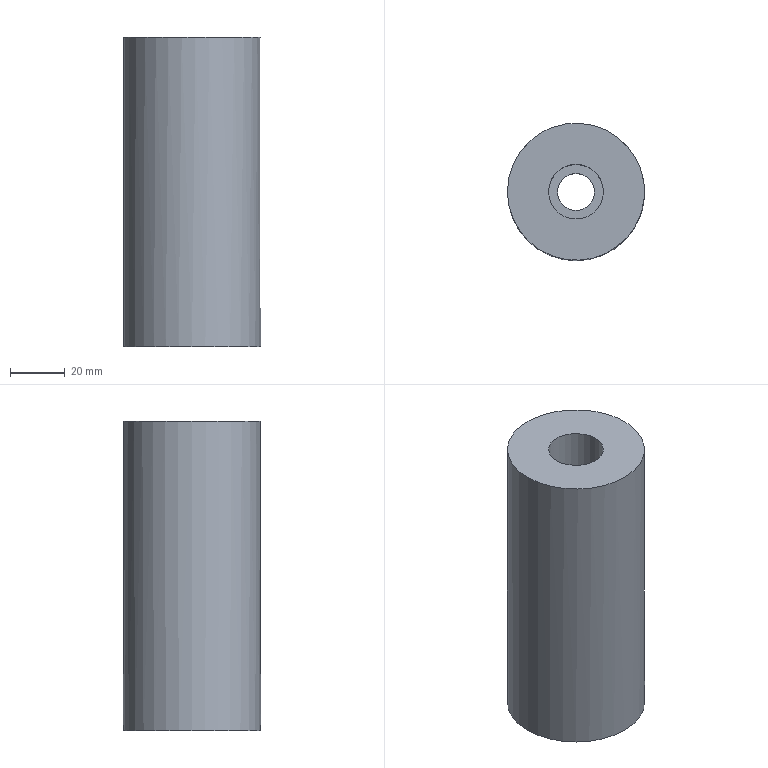Part | NX | features 27 2 | 1 solid | 6 faces | box 50 x 50 x 113 mm | volume 194926 mm3 | cylinder 3 | plane 3 | commonest cylinder face diameters 13.5 x1 20 x1 50 x1
STEP:
#1=CARTESIAN_POINT('',(27.,560.,-113.));
#2=VERTEX_POINT('',#1);
#3=CARTESIAN_POINT('',(2.,560.,-113.));
#4=DIRECTION('',(0.,0.,-1.));
#5=DIRECTION('',(1.,0.,0.));
#6=AXIS2_PLACEMENT_3D('',#3,#4,#5);
#7=CIRCLE('',#6,25.);
#8=EDGE_CURVE('',#2,#2,#7,.T.);
#9=ORIENTED_EDGE('',*,*,#8,.F.);
#10=EDGE_LOOP('',(#9));
#11=FACE_BOUND('',#10,.T.);
#12=CARTESIAN_POINT('',(-23.,560.,0.));
#13=VERTEX_POINT('',#12);
#14=CARTESIAN_POINT('',(2.,560.,0.));
#15=DIRECTION('',(0.,0.,-1.));
#16=DIRECTION('',(-1.,0.,0.));
#17=AXIS2_PLACEMENT_3D('',#14,#15,#16);
#18=CIRCLE('',#17,25.);
#19=EDGE_CURVE('',#13,#13,#18,.T.);
#20=ORIENTED_EDGE('',*,*,#19,.T.);
#21=EDGE_LOOP('',(#20));
#22=FACE_BOUND('',#21,.T.);
#23=CARTESIAN_POINT('',(2.,560.,30.));
#24=DIRECTION('',(0.,0.,1.));
#25=DIRECTION('',(-1.,0.,0.));
#26=AXIS2_PLACEMENT_3D('',#23,#24,#25);
#27=CYLINDRICAL_SURFACE('',#26,25.);
#28=ADVANCED_FACE('',(#11,#22),#27,.T.);
#29=CARTESIAN_POINT('',(12.,560.,-63.));
#30=VERTEX_POINT('',#29);
#31=CARTESIAN_POINT('',(2.,560.,-63.));
#32=DIRECTION('',(0.,0.,-1.));
#33=DIRECTION('',(1.,0.,0.));
#34=AXIS2_PLACEMENT_3D('',#31,#32,#33);
#35=CIRCLE('',#34,10.);
#36=EDGE_CURVE('',#30,#30,#35,.T.);
#37=ORIENTED_EDGE('',*,*,#36,.T.);
#38=EDGE_LOOP('',(#37));
#39=FACE_BOUND('',#38,.T.);
#40=CARTESIAN_POINT('',(-8.,560.,0.));
#41=VERTEX_POINT('',#40);
#42=CARTESIAN_POINT('',(2.,560.,0.));
#43=DIRECTION('',(0.,0.,1.));
#44=DIRECTION('',(-1.,0.,0.));
#45=AXIS2_PLACEMENT_3D('',#42,#43,#44);
#46=CIRCLE('',#45,10.);
#47=EDGE_CURVE('',#41,#41,#46,.T.);
#48=ORIENTED_EDGE('',*,*,#47,.T.);
#49=EDGE_LOOP('',(#48));
#50=FACE_BOUND('',#49,.T.);
#51=CARTESIAN_POINT('',(2.,560.,30.));
#52=DIRECTION('',(0.,0.,-1.));
#53=DIRECTION('',(1.,0.,0.));
#54=AXIS2_PLACEMENT_3D('',#51,#52,#53);
#55=CYLINDRICAL_SURFACE('',#54,10.);
#56=ADVANCED_FACE('',(#39,#50),#55,.F.);
#57=CARTESIAN_POINT('',(-4.75,560.,-63.));
#58=VERTEX_POINT('',#57);
#59=CARTESIAN_POINT('',(2.,560.,-63.));
#60=DIRECTION('',(0.,0.,-1.));
#61=DIRECTION('',(-1.,0.,0.));
#62=AXIS2_PLACEMENT_3D('',#59,#60,#61);
#63=CIRCLE('',#62,6.75);
#64=EDGE_CURVE('',#58,#58,#63,.T.);
#65=ORIENTED_EDGE('',*,*,#64,.F.);
#66=EDGE_LOOP('',(#65));
#67=FACE_BOUND('',#66,.T.);
#68=CARTESIAN_POINT('',(-4.75,560.,-113.));
#69=VERTEX_POINT('',#68);
#70=CARTESIAN_POINT('',(2.,560.,-113.));
#71=DIRECTION('',(0.,0.,-1.));
#72=DIRECTION('',(-1.,0.,0.));
#73=AXIS2_PLACEMENT_3D('',#70,#71,#72);
#74=CIRCLE('',#73,6.75);
#75=EDGE_CURVE('',#69,#69,#74,.T.);
#76=ORIENTED_EDGE('',*,*,#75,.T.);
#77=EDGE_LOOP('',(#76));
#78=FACE_BOUND('',#77,.T.);
#79=CARTESIAN_POINT('',(2.,560.,-5.));
#80=DIRECTION('',(0.,0.,-1.));
#81=DIRECTION('',(1.,0.,0.));
#82=AXIS2_PLACEMENT_3D('',#79,#80,#81);
#83=CYLINDRICAL_SURFACE('',#82,6.75);
#84=ADVANCED_FACE('',(#67,#78),#83,.F.);
#85=ORIENTED_EDGE('',*,*,#8,.T.);
#86=EDGE_LOOP('',(#85));
#87=FACE_BOUND('',#86,.T.);
#88=ORIENTED_EDGE('',*,*,#75,.F.);
#89=EDGE_LOOP('',(#88));
#90=FACE_BOUND('',#89,.T.);
#91=CARTESIAN_POINT('',(574.5,300.,-113.));
#92=DIRECTION('',(0.,0.,-1.));
#93=DIRECTION('',(1.,0.,0.));
#94=AXIS2_PLACEMENT_3D('',#91,#92,#93);
#95=PLANE('',#94);
#96=ADVANCED_FACE('',(#87,#90),#95,.T.);
#97=ORIENTED_EDGE('',*,*,#64,.T.);
#98=EDGE_LOOP('',(#97));
#99=FACE_BOUND('',#98,.T.);
#100=ORIENTED_EDGE('',*,*,#36,.F.);
#101=EDGE_LOOP('',(#100));
#102=FACE_BOUND('',#101,.T.);
#103=CARTESIAN_POINT('',(2.,560.,-63.));
#104=DIRECTION('',(0.,0.,-1.));
#105=DIRECTION('',(1.,0.,0.));
#106=AXIS2_PLACEMENT_3D('',#103,#104,#105);
#107=PLANE('',#106);
#108=ADVANCED_FACE('',(#99,#102),#107,.F.);
#109=ORIENTED_EDGE('',*,*,#47,.F.);
#110=EDGE_LOOP('',(#109));
#111=FACE_BOUND('',#110,.T.);
#112=ORIENTED_EDGE('',*,*,#19,.F.);
#113=EDGE_LOOP('',(#112));
#114=FACE_BOUND('',#113,.T.);
#115=CARTESIAN_POINT('',(340.,305.,0.));
#116=DIRECTION('',(0.,0.,1.));
#117=DIRECTION('',(-1.,0.,0.));
#118=AXIS2_PLACEMENT_3D('',#115,#116,#117);
#119=PLANE('',#118);
#120=ADVANCED_FACE('',(#111,#114),#119,.T.);
#121=CLOSED_SHELL('',(#28,#56,#84,#96,#108,#120));
#122=MANIFOLD_SOLID_BREP('',#121);
#123=(LENGTH_UNIT()NAMED_UNIT(*)SI_UNIT(.MILLI.,.METRE.));
#124=UNCERTAINTY_MEASURE_WITH_UNIT(LENGTH_MEASURE(0.00001),#123,'','');
#125=(NAMED_UNIT(*)PLANE_ANGLE_UNIT()SI_UNIT($,.RADIAN.));
#126=(NAMED_UNIT(*)SI_UNIT($,.STERADIAN.)SOLID_ANGLE_UNIT());
#127=(GEOMETRIC_REPRESENTATION_CONTEXT(3)GLOBAL_UNCERTAINTY_ASSIGNED_CONTEXT((#124))GLOBAL_UNIT_ASSIGNED_CONTEXT((#123,#125,#126))REPRESENTATION_CONTEXT('',''));
#128=ADVANCED_BREP_SHAPE_REPRESENTATION('',(#122),#127);